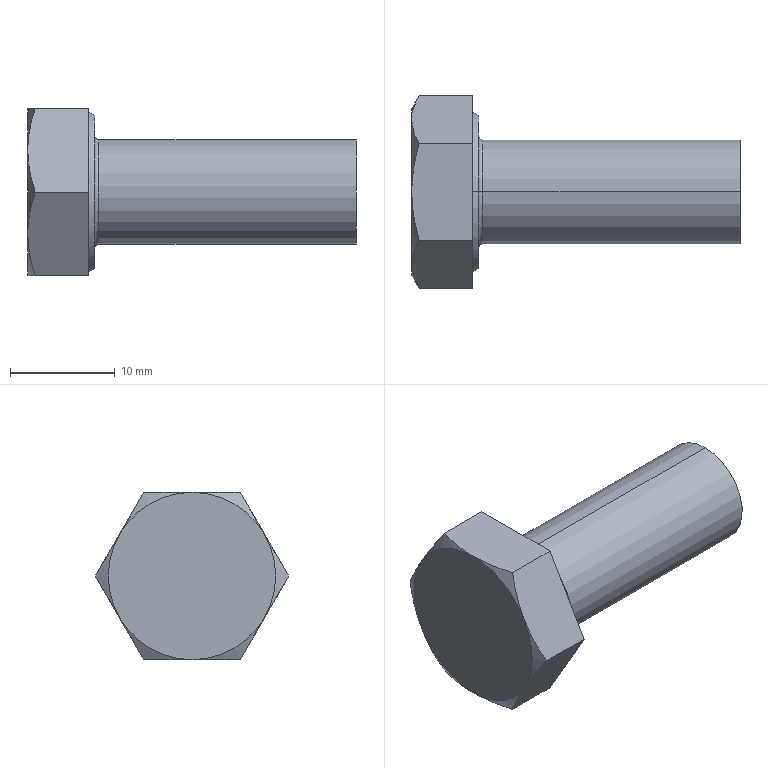Part | SolidWorks | features RevCut 3, Extrusion 1, Fillet 1, LPattern 1, Revolution 1 | 1 solid | 22 faces | box 31.4 x 18.475 x 16 mm | volume 3352 mm3 | plane 10 | cone 8 | torus 2 | cylinder 2 | commonest cylinder face diameters 10 x2
STEP:
#1=CARTESIAN_POINT('',(6.8,0.,5.));
#2=VERTEX_POINT('',#1);
#3=CARTESIAN_POINT('',(6.8,0.,-5.));
#4=VERTEX_POINT('',#3);
#5=CARTESIAN_POINT('',(6.8,0.,0.));
#6=DIRECTION('',(1.,0.,0.));
#7=DIRECTION('',(0.,0.,-1.));
#8=AXIS2_PLACEMENT_3D('',#5,#6,#7);
#9=CIRCLE('',#8,5.);
#10=EDGE_CURVE('',#2,#4,#9,.T.);
#11=ORIENTED_EDGE('',*,*,#10,.F.);
#12=CARTESIAN_POINT('',(6.4,0.,5.4));
#13=VERTEX_POINT('',#12);
#14=CARTESIAN_POINT('',(6.8,0.,5.4));
#15=DIRECTION('',(0.,1.,0.));
#16=DIRECTION('',(0.,0.,1.));
#17=AXIS2_PLACEMENT_3D('',#14,#15,#16);
#18=CIRCLE('',#17,0.4);
#19=EDGE_CURVE('',#2,#13,#18,.T.);
#20=ORIENTED_EDGE('',*,*,#19,.T.);
#21=CARTESIAN_POINT('',(6.4,0.,-5.4));
#22=VERTEX_POINT('',#21);
#23=CARTESIAN_POINT('',(6.4,0.,0.));
#24=DIRECTION('',(-1.,0.,0.));
#25=DIRECTION('',(0.,0.,-1.));
#26=AXIS2_PLACEMENT_3D('',#23,#24,#25);
#27=CIRCLE('',#26,5.4);
#28=EDGE_CURVE('',#22,#13,#27,.T.);
#29=ORIENTED_EDGE('',*,*,#28,.F.);
#30=CARTESIAN_POINT('',(6.8,0.,-5.4));
#31=DIRECTION('',(0.,-1.,0.));
#32=DIRECTION('',(0.,0.,-1.));
#33=AXIS2_PLACEMENT_3D('',#30,#31,#32);
#34=CIRCLE('',#33,0.4);
#35=EDGE_CURVE('',#4,#22,#34,.T.);
#36=ORIENTED_EDGE('',*,*,#35,.F.);
#37=EDGE_LOOP('',(#11,#20,#29,#36));
#38=FACE_OUTER_BOUND('',#37,.T.);
#39=CARTESIAN_POINT('',(6.8,0.,0.));
#40=DIRECTION('',(1.,0.,0.));
#41=DIRECTION('',(0.,0.,-1.));
#42=AXIS2_PLACEMENT_3D('',#39,#40,#41);
#43=TOROIDAL_SURFACE('',#42,5.4,0.4);
#44=ADVANCED_FACE('',(#38),#43,.F.);
#45=CARTESIAN_POINT('',(31.4,0.,5.));
#46=VERTEX_POINT('',#45);
#47=CARTESIAN_POINT('',(31.4,0.,-5.));
#48=VERTEX_POINT('',#47);
#49=CARTESIAN_POINT('',(31.4,0.,0.));
#50=DIRECTION('',(-1.,0.,0.));
#51=DIRECTION('',(0.,0.,1.));
#52=AXIS2_PLACEMENT_3D('',#49,#50,#51);
#53=CIRCLE('',#52,5.);
#54=EDGE_CURVE('',#46,#48,#53,.T.);
#55=ORIENTED_EDGE('',*,*,#54,.T.);
#56=CARTESIAN_POINT('',(0.,0.,-5.));
#57=DIRECTION('',(-1.,0.,0.));
#58=VECTOR('',#57,1000.);
#59=LINE('',#56,#58);
#60=EDGE_CURVE('',#48,#4,#59,.T.);
#61=ORIENTED_EDGE('',*,*,#60,.T.);
#62=CARTESIAN_POINT('',(6.8,0.,0.));
#63=DIRECTION('',(1.,0.,0.));
#64=DIRECTION('',(0.,0.,-1.));
#65=AXIS2_PLACEMENT_3D('',#62,#63,#64);
#66=CIRCLE('',#65,5.);
#67=EDGE_CURVE('',#4,#2,#66,.T.);
#68=ORIENTED_EDGE('',*,*,#67,.T.);
#69=CARTESIAN_POINT('',(0.,0.,5.));
#70=DIRECTION('',(-1.,0.,0.));
#71=VECTOR('',#70,1000.);
#72=LINE('',#69,#71);
#73=EDGE_CURVE('',#46,#2,#72,.T.);
#74=ORIENTED_EDGE('',*,*,#73,.F.);
#75=EDGE_LOOP('',(#55,#61,#68,#74));
#76=FACE_OUTER_BOUND('',#75,.T.);
#77=CARTESIAN_POINT('',(0.,0.,0.));
#78=DIRECTION('',(-1.,0.,0.));
#79=DIRECTION('',(0.,0.,1.));
#80=AXIS2_PLACEMENT_3D('',#77,#78,#79);
#81=CYLINDRICAL_SURFACE('',#80,5.);
#82=ADVANCED_FACE('',(#76),#81,.T.);
#83=CARTESIAN_POINT('',(6.4,0.,7.315));
#84=VERTEX_POINT('',#83);
#85=CARTESIAN_POINT('',(6.4,0.,-7.315));
#86=VERTEX_POINT('',#85);
#87=CARTESIAN_POINT('',(6.4,0.,0.));
#88=DIRECTION('',(-1.,0.,0.));
#89=DIRECTION('',(0.,0.,1.));
#90=AXIS2_PLACEMENT_3D('',#87,#88,#89);
#91=CIRCLE('',#90,7.315);
#92=EDGE_CURVE('',#84,#86,#91,.T.);
#93=ORIENTED_EDGE('',*,*,#92,.T.);
#94=CARTESIAN_POINT('',(5.8,0.,-7.661));
#95=VERTEX_POINT('',#94);
#96=CARTESIAN_POINT('',(5.8,0.,-7.661));
#97=DIRECTION('',(-0.866,0.,-0.5));
#98=VECTOR('',#97,1000.);
#99=LINE('',#96,#98);
#100=EDGE_CURVE('',#86,#95,#99,.T.);
#101=ORIENTED_EDGE('',*,*,#100,.T.);
#102=CARTESIAN_POINT('',(5.8,0.,7.661));
#103=VERTEX_POINT('',#102);
#104=CARTESIAN_POINT('',(5.8,0.,0.));
#105=DIRECTION('',(-1.,0.,0.));
#106=DIRECTION('',(0.,0.,1.));
#107=AXIS2_PLACEMENT_3D('',#104,#105,#106);
#108=CIRCLE('',#107,7.661);
#109=EDGE_CURVE('',#103,#95,#108,.T.);
#110=ORIENTED_EDGE('',*,*,#109,.F.);
#111=CARTESIAN_POINT('',(5.8,0.,7.661));
#112=DIRECTION('',(-0.866,0.,0.5));
#113=VECTOR('',#112,1000.);
#114=LINE('',#111,#113);
#115=EDGE_CURVE('',#84,#103,#114,.T.);
#116=ORIENTED_EDGE('',*,*,#115,.F.);
#117=EDGE_LOOP('',(#93,#101,#110,#116));
#118=FACE_OUTER_BOUND('',#117,.T.);
#119=CARTESIAN_POINT('',(5.8,0.,0.));
#120=DIRECTION('',(-1.,0.,0.));
#121=DIRECTION('',(0.,0.,1.));
#122=AXIS2_PLACEMENT_3D('',#119,#120,#121);
#123=CONICAL_SURFACE('',#122,7.661,0.5236);
#124=ADVANCED_FACE('',(#118),#123,.T.);
#125=CARTESIAN_POINT('',(5.8,4.619,-8.));
#126=VERTEX_POINT('',#125);
#127=CARTESIAN_POINT('',(5.8,9.238,0.));
#128=VERTEX_POINT('',#127);
#129=CARTESIAN_POINT('',(5.8,4.619,-8.));
#130=DIRECTION('',(0.,0.5,0.866));
#131=VECTOR('',#130,1000.);
#132=LINE('',#129,#131);
#133=EDGE_CURVE('',#126,#128,#132,.T.);
#134=ORIENTED_EDGE('',*,*,#133,.F.);
#135=CARTESIAN_POINT('',(0.7145,4.619,-8.));
#136=VERTEX_POINT('',#135);
#137=CARTESIAN_POINT('',(6.4,4.619,-8.));
#138=DIRECTION('',(-1.,0.,0.));
#139=VECTOR('',#138,1000.);
#140=LINE('',#137,#139);
#141=EDGE_CURVE('',#126,#136,#140,.T.);
#142=ORIENTED_EDGE('',*,*,#141,.T.);
#143=CARTESIAN_POINT('',(0.,6.928,-4.));
#144=VERTEX_POINT('',#143);
#145=CARTESIAN_POINT('',(0.,6.928,-4.));
#146=CARTESIAN_POINT('',(0.,6.732,-4.339));
#147=CARTESIAN_POINT('',(0.01689,6.535,-4.68));
#148=CARTESIAN_POINT('',(0.08225,6.146,-5.355));
#149=CARTESIAN_POINT('',(0.1307,5.952,-5.69));
#150=CARTESIAN_POINT('',(0.3174,5.376,-6.689));
#151=CARTESIAN_POINT('',(0.497,4.996,-7.347));
#152=CARTESIAN_POINT('',(0.7145,4.619,-8.));
#153=B_SPLINE_CURVE_WITH_KNOTS('',3,(#145,#146,#147,#148,#149,#150,#151,#152),.UNSPECIFIED.,.F.,.F.,(4,2,2,4),(0.004674,0.005838,0.007002,0.00933),.UNSPECIFIED.);
#154=EDGE_CURVE('',#144,#136,#153,.T.);
#155=ORIENTED_EDGE('',*,*,#154,.F.);
#156=CARTESIAN_POINT('',(0.7145,9.238,0.));
#157=VERTEX_POINT('',#156);
#158=CARTESIAN_POINT('',(0.7145,9.238,0.));
#159=CARTESIAN_POINT('',(0.4964,8.86,-0.6543));
#160=CARTESIAN_POINT('',(0.3167,8.479,-1.313));
#161=CARTESIAN_POINT('',(0.0681,7.71,-2.646));
#162=CARTESIAN_POINT('',(0.,7.322,-3.319));
#163=CARTESIAN_POINT('',(0.,6.928,-4.));
#164=B_SPLINE_CURVE_WITH_KNOTS('',3,(#158,#159,#160,#161,#162,#163),.UNSPECIFIED.,.F.,.F.,(4,2,4),(0.000000238,0.002337,0.004674),.UNSPECIFIED.);
#165=EDGE_CURVE('',#157,#144,#164,.T.);
#166=ORIENTED_EDGE('',*,*,#165,.F.);
#167=CARTESIAN_POINT('',(6.4,9.238,0.));
#168=DIRECTION('',(-1.,0.,0.));
#169=VECTOR('',#168,1000.);
#170=LINE('',#167,#169);
#171=EDGE_CURVE('',#128,#157,#170,.T.);
#172=ORIENTED_EDGE('',*,*,#171,.F.);
#173=EDGE_LOOP('',(#134,#142,#155,#166,#172));
#174=FACE_OUTER_BOUND('',#173,.T.);
#175=CARTESIAN_POINT('',(6.4,4.619,-8.));
#176=DIRECTION('',(0.,-0.866,0.5));
#177=DIRECTION('',(0.,-0.5,-0.866));
#178=AXIS2_PLACEMENT_3D('',#175,#176,#177);
#179=PLANE('',#178);
#180=ADVANCED_FACE('',(#174),#179,.F.);
#181=CARTESIAN_POINT('',(5.8,4.619,8.));
#182=VERTEX_POINT('',#181);
#183=CARTESIAN_POINT('',(5.8,9.238,0.));
#184=DIRECTION('',(0.,-0.5,0.866));
#185=VECTOR('',#184,1000.);
#186=LINE('',#183,#185);
#187=EDGE_CURVE('',#128,#182,#186,.T.);
#188=ORIENTED_EDGE('',*,*,#187,.F.);
#189=ORIENTED_EDGE('',*,*,#171,.T.);
#190=CARTESIAN_POINT('',(0.,6.928,4.));
#191=VERTEX_POINT('',#190);
#192=CARTESIAN_POINT('',(0.,6.928,4.));
#193=CARTESIAN_POINT('',(0.,7.124,3.661));
#194=CARTESIAN_POINT('',(0.01689,7.321,3.32));
#195=CARTESIAN_POINT('',(0.08225,7.711,2.645));
#196=CARTESIAN_POINT('',(0.1307,7.904,2.31));
#197=CARTESIAN_POINT('',(0.3174,8.481,1.311));
#198=CARTESIAN_POINT('',(0.497,8.861,0.6527));
#199=CARTESIAN_POINT('',(0.7145,9.238,0.));
#200=B_SPLINE_CURVE_WITH_KNOTS('',3,(#192,#193,#194,#195,#196,#197,#198,#199),.UNSPECIFIED.,.F.,.F.,(4,2,2,4),(0.004674,0.005838,0.007002,0.00933),.UNSPECIFIED.);
#201=EDGE_CURVE('',#191,#157,#200,.T.);
#202=ORIENTED_EDGE('',*,*,#201,.F.);
#203=CARTESIAN_POINT('',(0.7145,4.619,8.));
#204=VERTEX_POINT('',#203);
#205=CARTESIAN_POINT('',(0.7145,4.619,8.));
#206=CARTESIAN_POINT('',(0.4964,4.997,7.346));
#207=CARTESIAN_POINT('',(0.3167,5.377,6.687));
#208=CARTESIAN_POINT('',(0.0681,6.146,5.354));
#209=CARTESIAN_POINT('',(0.,6.535,4.681));
#210=CARTESIAN_POINT('',(0.,6.928,4.));
#211=B_SPLINE_CURVE_WITH_KNOTS('',3,(#205,#206,#207,#208,#209,#210),.UNSPECIFIED.,.F.,.F.,(4,2,4),(0.000000238,0.002337,0.004674),.UNSPECIFIED.);
#212=EDGE_CURVE('',#204,#191,#211,.T.);
#213=ORIENTED_EDGE('',*,*,#212,.F.);
#214=CARTESIAN_POINT('',(6.4,4.619,8.));
#215=DIRECTION('',(-1.,0.,0.));
#216=VECTOR('',#215,1000.);
#217=LINE('',#214,#216);
#218=EDGE_CURVE('',#182,#204,#217,.T.);
#219=ORIENTED_EDGE('',*,*,#218,.F.);
#220=EDGE_LOOP('',(#188,#189,#202,#213,#219));
#221=FACE_OUTER_BOUND('',#220,.T.);
#222=CARTESIAN_POINT('',(6.4,9.238,0.));
#223=DIRECTION('',(0.,-0.866,-0.5));
#224=DIRECTION('',(0.,0.5,-0.866));
#225=AXIS2_PLACEMENT_3D('',#222,#223,#224);
#226=PLANE('',#225);
#227=ADVANCED_FACE('',(#221),#226,.F.);
#228=CARTESIAN_POINT('',(5.8,-4.619,8.));
#229=VERTEX_POINT('',#228);
#230=CARTESIAN_POINT('',(5.8,4.619,8.));
#231=DIRECTION('',(0.,-1.,0.));
#232=VECTOR('',#231,1000.);
#233=LINE('',#230,#232);
#234=EDGE_CURVE('',#182,#229,#233,.T.);
#235=ORIENTED_EDGE('',*,*,#234,.F.);
#236=ORIENTED_EDGE('',*,*,#218,.T.);
#237=CARTESIAN_POINT('',(0.,0.,8.));
#238=VERTEX_POINT('',#237);
#239=CARTESIAN_POINT('',(0.,0.,8.));
#240=CARTESIAN_POINT('',(0.,0.3913,8.));
#241=CARTESIAN_POINT('',(0.01678,0.7854,8.));
#242=CARTESIAN_POINT('',(0.08286,1.571,8.));
#243=CARTESIAN_POINT('',(0.1318,1.96,8.));
#244=CARTESIAN_POINT('',(0.3194,3.115,8.));
#245=CARTESIAN_POINT('',(0.4988,3.872,8.));
#246=CARTESIAN_POINT('',(0.7145,4.619,8.));
#247=B_SPLINE_CURVE_WITH_KNOTS('',3,(#239,#240,#241,#242,#243,#244,#245,#246),.UNSPECIFIED.,.F.,.F.,(4,2,2,4),(0.01337,0.01454,0.01571,0.01805),.UNSPECIFIED.);
#248=EDGE_CURVE('',#238,#204,#247,.T.);
#249=ORIENTED_EDGE('',*,*,#248,.F.);
#250=CARTESIAN_POINT('',(0.7145,-4.619,8.));
#251=VERTEX_POINT('',#250);
#252=CARTESIAN_POINT('',(0.7145,-4.619,8.));
#253=CARTESIAN_POINT('',(0.4973,-3.866,8.));
#254=CARTESIAN_POINT('',(0.3158,-3.098,8.));
#255=CARTESIAN_POINT('',(0.0673,-1.557,8.));
#256=CARTESIAN_POINT('',(0.,-0.7819,8.));
#257=CARTESIAN_POINT('',(0.,0.,8.));
#258=B_SPLINE_CURVE_WITH_KNOTS('',3,(#252,#253,#254,#255,#256,#257),.UNSPECIFIED.,.F.,.F.,(4,2,4),(0.00869,0.01103,0.01337),.UNSPECIFIED.);
#259=EDGE_CURVE('',#251,#238,#258,.T.);
#260=ORIENTED_EDGE('',*,*,#259,.F.);
#261=CARTESIAN_POINT('',(6.4,-4.619,8.));
#262=DIRECTION('',(-1.,0.,0.));
#263=VECTOR('',#262,1000.);
#264=LINE('',#261,#263);
#265=EDGE_CURVE('',#229,#251,#264,.T.);
#266=ORIENTED_EDGE('',*,*,#265,.F.);
#267=EDGE_LOOP('',(#235,#236,#249,#260,#266));
#268=FACE_OUTER_BOUND('',#267,.T.);
#269=CARTESIAN_POINT('',(6.4,4.619,8.));
#270=DIRECTION('',(0.,0.,-1.));
#271=DIRECTION('',(0.,1.,0.));
#272=AXIS2_PLACEMENT_3D('',#269,#270,#271);
#273=PLANE('',#272);
#274=ADVANCED_FACE('',(#268),#273,.F.);
#275=CARTESIAN_POINT('',(5.8,-9.238,0.));
#276=VERTEX_POINT('',#275);
#277=CARTESIAN_POINT('',(5.8,-9.238,0.));
#278=DIRECTION('',(0.,-0.5,-0.866));
#279=VECTOR('',#278,1000.);
#280=LINE('',#277,#279);
#281=EDGE_CURVE('',#229,#276,#280,.T.);
#282=ORIENTED_EDGE('',*,*,#281,.F.);
#283=ORIENTED_EDGE('',*,*,#265,.T.);
#284=CARTESIAN_POINT('',(0.,-6.928,4.));
#285=VERTEX_POINT('',#284);
#286=CARTESIAN_POINT('',(0.,-6.928,4.));
#287=CARTESIAN_POINT('',(0.,-6.732,4.339));
#288=CARTESIAN_POINT('',(0.01689,-6.535,4.68));
#289=CARTESIAN_POINT('',(0.08225,-6.146,5.355));
#290=CARTESIAN_POINT('',(0.1307,-5.952,5.69));
#291=CARTESIAN_POINT('',(0.3174,-5.376,6.689));
#292=CARTESIAN_POINT('',(0.497,-4.996,7.347));
#293=CARTESIAN_POINT('',(0.7145,-4.619,8.));
#294=B_SPLINE_CURVE_WITH_KNOTS('',3,(#286,#287,#288,#289,#290,#291,#292,#293),.UNSPECIFIED.,.F.,.F.,(4,2,2,4),(0.004674,0.005838,0.007002,0.00933),.UNSPECIFIED.);
#295=EDGE_CURVE('',#285,#251,#294,.T.);
#296=ORIENTED_EDGE('',*,*,#295,.F.);
#297=CARTESIAN_POINT('',(0.7145,-9.238,0.));
#298=VERTEX_POINT('',#297);
#299=CARTESIAN_POINT('',(0.7145,-9.238,0.));
#300=CARTESIAN_POINT('',(0.4964,-8.86,0.6543));
#301=CARTESIAN_POINT('',(0.3167,-8.479,1.313));
#302=CARTESIAN_POINT('',(0.0681,-7.71,2.646));
#303=CARTESIAN_POINT('',(0.,-7.322,3.319));
#304=CARTESIAN_POINT('',(0.,-6.928,4.));
#305=B_SPLINE_CURVE_WITH_KNOTS('',3,(#299,#300,#301,#302,#303,#304),.UNSPECIFIED.,.F.,.F.,(4,2,4),(0.000000238,0.002337,0.004674),.UNSPECIFIED.);
#306=EDGE_CURVE('',#298,#285,#305,.T.);
#307=ORIENTED_EDGE('',*,*,#306,.F.);
#308=CARTESIAN_POINT('',(6.4,-9.238,0.));
#309=DIRECTION('',(-1.,0.,0.));
#310=VECTOR('',#309,1000.);
#311=LINE('',#308,#310);
#312=EDGE_CURVE('',#276,#298,#311,.T.);
#313=ORIENTED_EDGE('',*,*,#312,.F.);
#314=EDGE_LOOP('',(#282,#283,#296,#307,#313));
#315=FACE_OUTER_BOUND('',#314,.T.);
#316=CARTESIAN_POINT('',(6.4,-9.238,0.));
#317=DIRECTION('',(0.,0.866,-0.5));
#318=DIRECTION('',(0.,0.5,0.866));
#319=AXIS2_PLACEMENT_3D('',#316,#317,#318);
#320=PLANE('',#319);
#321=ADVANCED_FACE('',(#315),#320,.F.);
#322=CARTESIAN_POINT('',(5.8,-4.619,-8.));
#323=VERTEX_POINT('',#322);
#324=CARTESIAN_POINT('',(5.8,-4.619,-8.));
#325=DIRECTION('',(0.,0.5,-0.866));
#326=VECTOR('',#325,1000.);
#327=LINE('',#324,#326);
#328=EDGE_CURVE('',#276,#323,#327,.T.);
#329=ORIENTED_EDGE('',*,*,#328,.F.);
#330=ORIENTED_EDGE('',*,*,#312,.T.);
#331=CARTESIAN_POINT('',(0.,-6.928,-4.));
#332=VERTEX_POINT('',#331);
#333=CARTESIAN_POINT('',(0.,-6.928,-4.));
#334=CARTESIAN_POINT('',(0.,-7.124,-3.661));
#335=CARTESIAN_POINT('',(0.01689,-7.321,-3.32));
#336=CARTESIAN_POINT('',(0.08225,-7.711,-2.645));
#337=CARTESIAN_POINT('',(0.1307,-7.904,-2.31));
#338=CARTESIAN_POINT('',(0.3174,-8.481,-1.311));
#339=CARTESIAN_POINT('',(0.497,-8.861,-0.6527));
#340=CARTESIAN_POINT('',(0.7145,-9.238,0.));
#341=B_SPLINE_CURVE_WITH_KNOTS('',3,(#333,#334,#335,#336,#337,#338,#339,#340),.UNSPECIFIED.,.F.,.F.,(4,2,2,4),(0.004674,0.005838,0.007002,0.00933),.UNSPECIFIED.);
#342=EDGE_CURVE('',#332,#298,#341,.T.);
#343=ORIENTED_EDGE('',*,*,#342,.F.);
#344=CARTESIAN_POINT('',(0.7145,-4.619,-8.));
#345=VERTEX_POINT('',#344);
#346=CARTESIAN_POINT('',(0.7145,-4.619,-8.));
#347=CARTESIAN_POINT('',(0.4964,-4.997,-7.346));
#348=CARTESIAN_POINT('',(0.3167,-5.377,-6.687));
#349=CARTESIAN_POINT('',(0.0681,-6.146,-5.354));
#350=CARTESIAN_POINT('',(0.,-6.535,-4.681));
#351=CARTESIAN_POINT('',(0.,-6.928,-4.));
#352=B_SPLINE_CURVE_WITH_KNOTS('',3,(#346,#347,#348,#349,#350,#351),.UNSPECIFIED.,.F.,.F.,(4,2,4),(0.000000238,0.002337,0.004674),.UNSPECIFIED.);
#353=EDGE_CURVE('',#345,#332,#352,.T.);
#354=ORIENTED_EDGE('',*,*,#353,.F.);
#355=CARTESIAN_POINT('',(6.4,-4.619,-8.));
#356=DIRECTION('',(-1.,0.,0.));
#357=VECTOR('',#356,1000.);
#358=LINE('',#355,#357);
#359=EDGE_CURVE('',#323,#345,#358,.T.);
#360=ORIENTED_EDGE('',*,*,#359,.F.);
#361=EDGE_LOOP('',(#329,#330,#343,#354,#360));
#362=FACE_OUTER_BOUND('',#361,.T.);
#363=CARTESIAN_POINT('',(6.4,-4.619,-8.));
#364=DIRECTION('',(0.,0.866,0.5));
#365=DIRECTION('',(0.,-0.5,0.866));
#366=AXIS2_PLACEMENT_3D('',#363,#364,#365);
#367=PLANE('',#366);
#368=ADVANCED_FACE('',(#362),#367,.F.);
#369=CARTESIAN_POINT('',(5.8,4.619,-8.));
#370=DIRECTION('',(0.,1.,0.));
#371=VECTOR('',#370,1000.);
#372=LINE('',#369,#371);
#373=EDGE_CURVE('',#323,#126,#372,.T.);
#374=ORIENTED_EDGE('',*,*,#373,.F.);
#375=ORIENTED_EDGE('',*,*,#359,.T.);
#376=CARTESIAN_POINT('',(0.,0.,-8.));
#377=VERTEX_POINT('',#376);
#378=CARTESIAN_POINT('',(0.,0.,-8.));
#379=CARTESIAN_POINT('',(0.,-0.7819,-8.));
#380=CARTESIAN_POINT('',(0.0673,-1.557,-8.));
#381=CARTESIAN_POINT('',(0.3158,-3.098,-8.));
#382=CARTESIAN_POINT('',(0.4973,-3.866,-8.));
#383=CARTESIAN_POINT('',(0.7145,-4.619,-8.));
#384=B_SPLINE_CURVE_WITH_KNOTS('',3,(#378,#379,#380,#381,#382,#383),.UNSPECIFIED.,.F.,.F.,(4,2,4),(0.02753,0.02987,0.03221),.UNSPECIFIED.);
#385=EDGE_CURVE('',#377,#345,#384,.T.);
#386=ORIENTED_EDGE('',*,*,#385,.F.);
#387=CARTESIAN_POINT('',(0.7145,4.619,-8.));
#388=CARTESIAN_POINT('',(0.4988,3.872,-8.));
#389=CARTESIAN_POINT('',(0.3194,3.115,-8.));
#390=CARTESIAN_POINT('',(0.1318,1.96,-8.));
#391=CARTESIAN_POINT('',(0.08286,1.571,-8.));
#392=CARTESIAN_POINT('',(0.01678,0.7854,-8.));
#393=CARTESIAN_POINT('',(0.,0.3913,-8.));
#394=CARTESIAN_POINT('',(0.,0.,-8.));
#395=B_SPLINE_CURVE_WITH_KNOTS('',3,(#387,#388,#389,#390,#391,#392,#393,#394),.UNSPECIFIED.,.F.,.F.,(4,2,2,4),(0.02285,0.02519,0.02636,0.02753),.UNSPECIFIED.);
#396=EDGE_CURVE('',#136,#377,#395,.T.);
#397=ORIENTED_EDGE('',*,*,#396,.F.);
#398=ORIENTED_EDGE('',*,*,#141,.F.);
#399=EDGE_LOOP('',(#374,#375,#386,#397,#398));
#400=FACE_OUTER_BOUND('',#399,.T.);
#401=CARTESIAN_POINT('',(6.4,4.619,-8.));
#402=DIRECTION('',(0.,0.,1.));
#403=DIRECTION('',(1.,0.,0.));
#404=AXIS2_PLACEMENT_3D('',#401,#402,#403);
#405=PLANE('',#404);
#406=ADVANCED_FACE('',(#400),#405,.F.);
#407=ORIENTED_EDGE('',*,*,#353,.T.);
#408=CARTESIAN_POINT('',(0.,0.,0.));
#409=DIRECTION('',(1.,0.,0.));
#410=DIRECTION('',(0.,0.,-1.));
#411=AXIS2_PLACEMENT_3D('',#408,#409,#410);
#412=CIRCLE('',#411,8.);
#413=EDGE_CURVE('',#332,#377,#412,.T.);
#414=ORIENTED_EDGE('',*,*,#413,.T.);
#415=ORIENTED_EDGE('',*,*,#385,.T.);
#416=EDGE_LOOP('',(#407,#414,#415));
#417=FACE_OUTER_BOUND('',#416,.T.);
#418=CARTESIAN_POINT('',(0.,0.,0.));
#419=DIRECTION('',(1.,0.,0.));
#420=DIRECTION('',(0.,0.,-1.));
#421=AXIS2_PLACEMENT_3D('',#418,#419,#420);
#422=CONICAL_SURFACE('',#421,8.,1.047);
#423=ADVANCED_FACE('',(#417),#422,.T.);
#424=ORIENTED_EDGE('',*,*,#306,.T.);
#425=CARTESIAN_POINT('',(0.,0.,0.));
#426=DIRECTION('',(1.,0.,0.));
#427=DIRECTION('',(0.,0.,-1.));
#428=AXIS2_PLACEMENT_3D('',#425,#426,#427);
#429=CIRCLE('',#428,8.);
#430=EDGE_CURVE('',#285,#332,#429,.T.);
#431=ORIENTED_EDGE('',*,*,#430,.T.);
#432=ORIENTED_EDGE('',*,*,#342,.T.);
#433=EDGE_LOOP('',(#424,#431,#432));
#434=FACE_OUTER_BOUND('',#433,.T.);
#435=CARTESIAN_POINT('',(0.,0.,0.));
#436=DIRECTION('',(1.,0.,0.));
#437=DIRECTION('',(0.,0.,-1.));
#438=AXIS2_PLACEMENT_3D('',#435,#436,#437);
#439=CONICAL_SURFACE('',#438,8.,1.047);
#440=ADVANCED_FACE('',(#434),#439,.T.);
#441=ORIENTED_EDGE('',*,*,#259,.T.);
#442=CARTESIAN_POINT('',(0.,0.,0.));
#443=DIRECTION('',(1.,0.,0.));
#444=DIRECTION('',(0.,0.,-1.));
#445=AXIS2_PLACEMENT_3D('',#442,#443,#444);
#446=CIRCLE('',#445,8.);
#447=EDGE_CURVE('',#238,#285,#446,.T.);
#448=ORIENTED_EDGE('',*,*,#447,.T.);
#449=ORIENTED_EDGE('',*,*,#295,.T.);
#450=EDGE_LOOP('',(#441,#448,#449));
#451=FACE_OUTER_BOUND('',#450,.T.);
#452=CARTESIAN_POINT('',(0.,0.,0.));
#453=DIRECTION('',(1.,0.,0.));
#454=DIRECTION('',(0.,0.,-1.));
#455=AXIS2_PLACEMENT_3D('',#452,#453,#454);
#456=CONICAL_SURFACE('',#455,8.,1.047);
#457=ADVANCED_FACE('',(#451),#456,.T.);
#458=ORIENTED_EDGE('',*,*,#248,.T.);
#459=ORIENTED_EDGE('',*,*,#212,.T.);
#460=CARTESIAN_POINT('',(0.,0.,0.));
#461=DIRECTION('',(-1.,0.,0.));
#462=DIRECTION('',(0.,0.,1.));
#463=AXIS2_PLACEMENT_3D('',#460,#461,#462);
#464=CIRCLE('',#463,8.);
#465=EDGE_CURVE('',#238,#191,#464,.T.);
#466=ORIENTED_EDGE('',*,*,#465,.F.);
#467=EDGE_LOOP('',(#458,#459,#466));
#468=FACE_OUTER_BOUND('',#467,.T.);
#469=CARTESIAN_POINT('',(0.,0.,0.));
#470=DIRECTION('',(1.,0.,0.));
#471=DIRECTION('',(0.,0.,-1.));
#472=AXIS2_PLACEMENT_3D('',#469,#470,#471);
#473=CONICAL_SURFACE('',#472,8.,1.047);
#474=ADVANCED_FACE('',(#468),#473,.T.);
#475=ORIENTED_EDGE('',*,*,#201,.T.);
#476=ORIENTED_EDGE('',*,*,#165,.T.);
#477=CARTESIAN_POINT('',(0.,0.,0.));
#478=DIRECTION('',(1.,0.,0.));
#479=DIRECTION('',(0.,0.,-1.));
#480=AXIS2_PLACEMENT_3D('',#477,#478,#479);
#481=CIRCLE('',#480,8.);
#482=EDGE_CURVE('',#144,#191,#481,.T.);
#483=ORIENTED_EDGE('',*,*,#482,.T.);
#484=EDGE_LOOP('',(#475,#476,#483));
#485=FACE_OUTER_BOUND('',#484,.T.);
#486=CARTESIAN_POINT('',(0.,0.,0.));
#487=DIRECTION('',(1.,0.,0.));
#488=DIRECTION('',(0.,0.,-1.));
#489=AXIS2_PLACEMENT_3D('',#486,#487,#488);
#490=CONICAL_SURFACE('',#489,8.,1.047);
#491=ADVANCED_FACE('',(#485),#490,.T.);
#492=ORIENTED_EDGE('',*,*,#154,.T.);
#493=ORIENTED_EDGE('',*,*,#396,.T.);
#494=CARTESIAN_POINT('',(0.,0.,0.));
#495=DIRECTION('',(1.,0.,0.));
#496=DIRECTION('',(0.,0.,-1.));
#497=AXIS2_PLACEMENT_3D('',#494,#495,#496);
#498=CIRCLE('',#497,8.);
#499=EDGE_CURVE('',#377,#144,#498,.T.);
#500=ORIENTED_EDGE('',*,*,#499,.T.);
#501=EDGE_LOOP('',(#492,#493,#500));
#502=FACE_OUTER_BOUND('',#501,.T.);
#503=CARTESIAN_POINT('',(0.,0.,0.));
#504=DIRECTION('',(1.,0.,0.));
#505=DIRECTION('',(0.,0.,-1.));
#506=AXIS2_PLACEMENT_3D('',#503,#504,#505);
#507=CONICAL_SURFACE('',#506,8.,1.047);
#508=ADVANCED_FACE('',(#502),#507,.T.);
#509=ORIENTED_EDGE('',*,*,#499,.F.);
#510=ORIENTED_EDGE('',*,*,#413,.F.);
#511=ORIENTED_EDGE('',*,*,#430,.F.);
#512=ORIENTED_EDGE('',*,*,#447,.F.);
#513=ORIENTED_EDGE('',*,*,#465,.T.);
#514=ORIENTED_EDGE('',*,*,#482,.F.);
#515=EDGE_LOOP('',(#509,#510,#511,#512,#513,#514));
#516=FACE_OUTER_BOUND('',#515,.T.);
#517=CARTESIAN_POINT('',(0.,9.238,0.));
#518=DIRECTION('',(1.,0.,0.));
#519=DIRECTION('',(0.,0.,-1.));
#520=AXIS2_PLACEMENT_3D('',#517,#518,#519);
#521=PLANE('',#520);
#522=ADVANCED_FACE('',(#516),#521,.F.);
#523=ORIENTED_EDGE('',*,*,#109,.T.);
#524=CARTESIAN_POINT('',(5.8,0.,0.));
#525=DIRECTION('',(-1.,0.,0.));
#526=DIRECTION('',(0.,0.,1.));
#527=AXIS2_PLACEMENT_3D('',#524,#525,#526);
#528=CIRCLE('',#527,7.661);
#529=EDGE_CURVE('',#95,#103,#528,.T.);
#530=ORIENTED_EDGE('',*,*,#529,.T.);
#531=EDGE_LOOP('',(#523,#530));
#532=FACE_BOUND('',#531,.T.);
#533=ORIENTED_EDGE('',*,*,#133,.T.);
#534=ORIENTED_EDGE('',*,*,#187,.T.);
#535=ORIENTED_EDGE('',*,*,#234,.T.);
#536=ORIENTED_EDGE('',*,*,#281,.T.);
#537=ORIENTED_EDGE('',*,*,#328,.T.);
#538=ORIENTED_EDGE('',*,*,#373,.T.);
#539=EDGE_LOOP('',(#533,#534,#535,#536,#537,#538));
#540=FACE_OUTER_BOUND('',#539,.T.);
#541=CARTESIAN_POINT('',(5.8,7.661,0.));
#542=DIRECTION('',(1.,0.,0.));
#543=DIRECTION('',(0.,0.,-1.));
#544=AXIS2_PLACEMENT_3D('',#541,#542,#543);
#545=PLANE('',#544);
#546=ADVANCED_FACE('',(#532,#540),#545,.T.);
#547=ORIENTED_EDGE('',*,*,#100,.F.);
#548=CARTESIAN_POINT('',(6.4,0.,0.));
#549=DIRECTION('',(-1.,0.,0.));
#550=DIRECTION('',(0.,0.,1.));
#551=AXIS2_PLACEMENT_3D('',#548,#549,#550);
#552=CIRCLE('',#551,7.315);
#553=EDGE_CURVE('',#86,#84,#552,.T.);
#554=ORIENTED_EDGE('',*,*,#553,.T.);
#555=ORIENTED_EDGE('',*,*,#115,.T.);
#556=ORIENTED_EDGE('',*,*,#529,.F.);
#557=EDGE_LOOP('',(#547,#554,#555,#556));
#558=FACE_OUTER_BOUND('',#557,.T.);
#559=CARTESIAN_POINT('',(5.8,0.,0.));
#560=DIRECTION('',(-1.,0.,0.));
#561=DIRECTION('',(0.,0.,1.));
#562=AXIS2_PLACEMENT_3D('',#559,#560,#561);
#563=CONICAL_SURFACE('',#562,7.661,0.5236);
#564=ADVANCED_FACE('',(#558),#563,.T.);
#565=ORIENTED_EDGE('',*,*,#54,.F.);
#566=CARTESIAN_POINT('',(31.4,0.,0.));
#567=DIRECTION('',(-1.,0.,0.));
#568=DIRECTION('',(0.,0.,1.));
#569=AXIS2_PLACEMENT_3D('',#566,#567,#568);
#570=CIRCLE('',#569,5.);
#571=EDGE_CURVE('',#48,#46,#570,.T.);
#572=ORIENTED_EDGE('',*,*,#571,.F.);
#573=EDGE_LOOP('',(#565,#572));
#574=FACE_OUTER_BOUND('',#573,.T.);
#575=CARTESIAN_POINT('',(31.4,0.,0.));
#576=DIRECTION('',(-1.,0.,0.));
#577=DIRECTION('',(0.,0.,1.));
#578=AXIS2_PLACEMENT_3D('',#575,#576,#577);
#579=PLANE('',#578);
#580=ADVANCED_FACE('',(#574),#579,.F.);
#581=ORIENTED_EDGE('',*,*,#60,.F.);
#582=ORIENTED_EDGE('',*,*,#571,.T.);
#583=ORIENTED_EDGE('',*,*,#73,.T.);
#584=ORIENTED_EDGE('',*,*,#10,.T.);
#585=EDGE_LOOP('',(#581,#582,#583,#584));
#586=FACE_OUTER_BOUND('',#585,.T.);
#587=CARTESIAN_POINT('',(0.,0.,0.));
#588=DIRECTION('',(-1.,0.,0.));
#589=DIRECTION('',(0.,0.,1.));
#590=AXIS2_PLACEMENT_3D('',#587,#588,#589);
#591=CYLINDRICAL_SURFACE('',#590,5.);
#592=ADVANCED_FACE('',(#586),#591,.T.);
#593=ORIENTED_EDGE('',*,*,#28,.T.);
#594=CARTESIAN_POINT('',(6.4,0.,0.));
#595=DIRECTION('',(-1.,0.,0.));
#596=DIRECTION('',(0.,0.,-1.));
#597=AXIS2_PLACEMENT_3D('',#594,#595,#596);
#598=CIRCLE('',#597,5.4);
#599=EDGE_CURVE('',#13,#22,#598,.T.);
#600=ORIENTED_EDGE('',*,*,#599,.T.);
#601=EDGE_LOOP('',(#593,#600));
#602=FACE_BOUND('',#601,.T.);
#603=ORIENTED_EDGE('',*,*,#92,.F.);
#604=ORIENTED_EDGE('',*,*,#553,.F.);
#605=EDGE_LOOP('',(#603,#604));
#606=FACE_OUTER_BOUND('',#605,.T.);
#607=CARTESIAN_POINT('',(6.4,9.238,0.));
#608=DIRECTION('',(1.,0.,0.));
#609=DIRECTION('',(0.,0.,-1.));
#610=AXIS2_PLACEMENT_3D('',#607,#608,#609);
#611=PLANE('',#610);
#612=ADVANCED_FACE('',(#602,#606),#611,.T.);
#613=ORIENTED_EDGE('',*,*,#19,.F.);
#614=ORIENTED_EDGE('',*,*,#67,.F.);
#615=ORIENTED_EDGE('',*,*,#35,.T.);
#616=ORIENTED_EDGE('',*,*,#599,.F.);
#617=EDGE_LOOP('',(#613,#614,#615,#616));
#618=FACE_OUTER_BOUND('',#617,.T.);
#619=CARTESIAN_POINT('',(6.8,0.,0.));
#620=DIRECTION('',(1.,0.,0.));
#621=DIRECTION('',(0.,0.,-1.));
#622=AXIS2_PLACEMENT_3D('',#619,#620,#621);
#623=TOROIDAL_SURFACE('',#622,5.4,0.4);
#624=ADVANCED_FACE('',(#618),#623,.F.);
#625=CLOSED_SHELL('',(#44,#82,#124,#180,#227,#274,#321,#368,#406,#423,#440,#457,#474,#491,#508,#522,#546,#564,#580,#592,#612,#624));
#626=MANIFOLD_SOLID_BREP('',#625);
#627=CARTESIAN_POINT('',(0.,0.,0.));
#628=DIRECTION('',(0.,0.,1.));
#629=DIRECTION('',(1.,0.,0.));
#630=AXIS2_PLACEMENT_3D('',#627,#628,#629);
#631=(LENGTH_UNIT()NAMED_UNIT(*)SI_UNIT(.MILLI.,.METRE.));
#632=UNCERTAINTY_MEASURE_WITH_UNIT(LENGTH_MEASURE(0.00001),#631,'','');
#633=(NAMED_UNIT(*)PLANE_ANGLE_UNIT()SI_UNIT($,.RADIAN.));
#634=(NAMED_UNIT(*)SI_UNIT($,.STERADIAN.)SOLID_ANGLE_UNIT());
#635=(GEOMETRIC_REPRESENTATION_CONTEXT(3)GLOBAL_UNCERTAINTY_ASSIGNED_CONTEXT((#632))GLOBAL_UNIT_ASSIGNED_CONTEXT((#631,#633,#634))REPRESENTATION_CONTEXT('',''));
#636=ADVANCED_BREP_SHAPE_REPRESENTATION('',(#626,#630),#635);